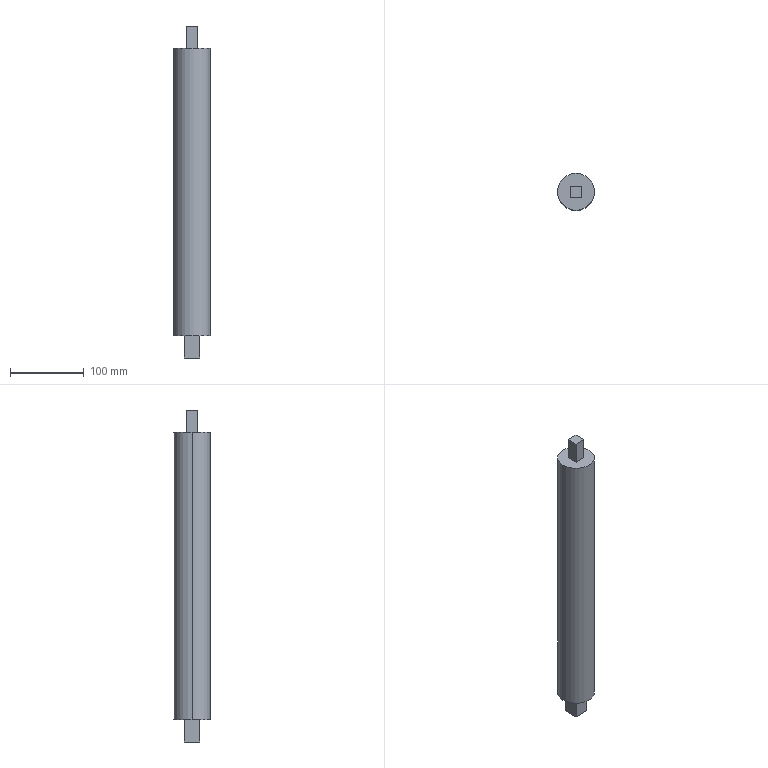Part | SolidWorks | features Extrusion 1, ICE 1, MoveFace 1 | 1 solid | 14 faces | box 50 x 50 x 450 mm | volume 785743 mm3 | plane 12 | cylinder 2 | commonest cylinder face diameters 50 x2
STEP:
#1=CARTESIAN_POINT('',(25.,0.,195.));
#2=VERTEX_POINT('',#1);
#3=CARTESIAN_POINT('',(-25.,0.,195.));
#4=VERTEX_POINT('',#3);
#5=CARTESIAN_POINT('',(0.,0.,195.));
#6=DIRECTION('',(0.,0.,1.));
#7=DIRECTION('',(1.,0.,0.));
#8=AXIS2_PLACEMENT_3D('',#5,#6,#7);
#9=CIRCLE('',#8,25.);
#10=EDGE_CURVE('',#2,#4,#9,.T.);
#11=ORIENTED_EDGE('',*,*,#10,.F.);
#12=CARTESIAN_POINT('',(25.,0.,-195.));
#13=VERTEX_POINT('',#12);
#14=CARTESIAN_POINT('',(25.,0.,195.));
#15=DIRECTION('',(0.,0.,-1.));
#16=VECTOR('',#15,1000.);
#17=LINE('',#14,#16);
#18=EDGE_CURVE('',#2,#13,#17,.T.);
#19=ORIENTED_EDGE('',*,*,#18,.T.);
#20=CARTESIAN_POINT('',(-25.,0.,-195.));
#21=VERTEX_POINT('',#20);
#22=CARTESIAN_POINT('',(0.,0.,-195.));
#23=DIRECTION('',(0.,0.,1.));
#24=DIRECTION('',(1.,0.,0.));
#25=AXIS2_PLACEMENT_3D('',#22,#23,#24);
#26=CIRCLE('',#25,25.);
#27=EDGE_CURVE('',#13,#21,#26,.T.);
#28=ORIENTED_EDGE('',*,*,#27,.T.);
#29=CARTESIAN_POINT('',(-25.,0.,195.));
#30=DIRECTION('',(0.,0.,-1.));
#31=VECTOR('',#30,1000.);
#32=LINE('',#29,#31);
#33=EDGE_CURVE('',#4,#21,#32,.T.);
#34=ORIENTED_EDGE('',*,*,#33,.F.);
#35=EDGE_LOOP('',(#11,#19,#28,#34));
#36=FACE_OUTER_BOUND('',#35,.T.);
#37=CARTESIAN_POINT('',(0.,0.,195.));
#38=DIRECTION('',(0.,0.,-1.));
#39=DIRECTION('',(-1.,0.,0.));
#40=AXIS2_PLACEMENT_3D('',#37,#38,#39);
#41=CYLINDRICAL_SURFACE('',#40,25.);
#42=ADVANCED_FACE('',(#36),#41,.T.);
#43=CARTESIAN_POINT('',(0.,0.,195.));
#44=DIRECTION('',(0.,0.,1.));
#45=DIRECTION('',(1.,0.,0.));
#46=AXIS2_PLACEMENT_3D('',#43,#44,#45);
#47=CIRCLE('',#46,25.);
#48=EDGE_CURVE('',#4,#2,#47,.T.);
#49=ORIENTED_EDGE('',*,*,#48,.T.);
#50=ORIENTED_EDGE('',*,*,#10,.T.);
#51=EDGE_LOOP('',(#49,#50));
#52=FACE_OUTER_BOUND('',#51,.T.);
#53=CARTESIAN_POINT('',(-7.5,7.5,195.));
#54=VERTEX_POINT('',#53);
#55=CARTESIAN_POINT('',(7.5,7.5,195.));
#56=VERTEX_POINT('',#55);
#57=CARTESIAN_POINT('',(0.,7.5,195.));
#58=DIRECTION('',(1.,0.,0.));
#59=VECTOR('',#58,1000.);
#60=LINE('',#57,#59);
#61=EDGE_CURVE('',#54,#56,#60,.T.);
#62=ORIENTED_EDGE('',*,*,#61,.T.);
#63=CARTESIAN_POINT('',(7.5,-7.5,195.));
#64=VERTEX_POINT('',#63);
#65=CARTESIAN_POINT('',(7.5,0.,195.));
#66=DIRECTION('',(0.,-1.,0.));
#67=VECTOR('',#66,1000.);
#68=LINE('',#65,#67);
#69=EDGE_CURVE('',#56,#64,#68,.T.);
#70=ORIENTED_EDGE('',*,*,#69,.T.);
#71=CARTESIAN_POINT('',(-7.5,-7.5,195.));
#72=VERTEX_POINT('',#71);
#73=CARTESIAN_POINT('',(0.,-7.5,195.));
#74=DIRECTION('',(-1.,0.,0.));
#75=VECTOR('',#74,1000.);
#76=LINE('',#73,#75);
#77=EDGE_CURVE('',#64,#72,#76,.T.);
#78=ORIENTED_EDGE('',*,*,#77,.T.);
#79=CARTESIAN_POINT('',(-7.5,0.,195.));
#80=DIRECTION('',(0.,1.,0.));
#81=VECTOR('',#80,1000.);
#82=LINE('',#79,#81);
#83=EDGE_CURVE('',#72,#54,#82,.T.);
#84=ORIENTED_EDGE('',*,*,#83,.T.);
#85=EDGE_LOOP('',(#62,#70,#78,#84));
#86=FACE_BOUND('',#85,.T.);
#87=CARTESIAN_POINT('',(0.,0.,195.));
#88=DIRECTION('',(0.,0.,1.));
#89=DIRECTION('',(1.,0.,0.));
#90=AXIS2_PLACEMENT_3D('',#87,#88,#89);
#91=PLANE('',#90);
#92=ADVANCED_FACE('',(#52,#86),#91,.T.);
#93=CARTESIAN_POINT('',(0.,0.,-195.));
#94=DIRECTION('',(0.,0.,1.));
#95=DIRECTION('',(1.,0.,0.));
#96=AXIS2_PLACEMENT_3D('',#93,#94,#95);
#97=CIRCLE('',#96,25.);
#98=EDGE_CURVE('',#21,#13,#97,.T.);
#99=ORIENTED_EDGE('',*,*,#98,.F.);
#100=ORIENTED_EDGE('',*,*,#27,.F.);
#101=EDGE_LOOP('',(#99,#100));
#102=FACE_OUTER_BOUND('',#101,.T.);
#103=CARTESIAN_POINT('',(10.5,10.5,-195.));
#104=VERTEX_POINT('',#103);
#105=CARTESIAN_POINT('',(10.5,-10.5,-195.));
#106=VERTEX_POINT('',#105);
#107=CARTESIAN_POINT('',(10.5,0.,-195.));
#108=DIRECTION('',(0.,-1.,0.));
#109=VECTOR('',#108,1000.);
#110=LINE('',#107,#109);
#111=EDGE_CURVE('',#104,#106,#110,.T.);
#112=ORIENTED_EDGE('',*,*,#111,.F.);
#113=CARTESIAN_POINT('',(-10.5,10.5,-195.));
#114=VERTEX_POINT('',#113);
#115=CARTESIAN_POINT('',(0.,10.5,-195.));
#116=DIRECTION('',(1.,0.,0.));
#117=VECTOR('',#116,1000.);
#118=LINE('',#115,#117);
#119=EDGE_CURVE('',#114,#104,#118,.T.);
#120=ORIENTED_EDGE('',*,*,#119,.F.);
#121=CARTESIAN_POINT('',(-10.5,-10.5,-195.));
#122=VERTEX_POINT('',#121);
#123=CARTESIAN_POINT('',(-10.5,0.,-195.));
#124=DIRECTION('',(0.,1.,0.));
#125=VECTOR('',#124,1000.);
#126=LINE('',#123,#125);
#127=EDGE_CURVE('',#122,#114,#126,.T.);
#128=ORIENTED_EDGE('',*,*,#127,.F.);
#129=CARTESIAN_POINT('',(0.,-10.5,-195.));
#130=DIRECTION('',(-1.,0.,0.));
#131=VECTOR('',#130,1000.);
#132=LINE('',#129,#131);
#133=EDGE_CURVE('',#106,#122,#132,.T.);
#134=ORIENTED_EDGE('',*,*,#133,.F.);
#135=EDGE_LOOP('',(#112,#120,#128,#134));
#136=FACE_BOUND('',#135,.T.);
#137=CARTESIAN_POINT('',(0.,0.,-195.));
#138=DIRECTION('',(0.,0.,1.));
#139=DIRECTION('',(1.,0.,0.));
#140=AXIS2_PLACEMENT_3D('',#137,#138,#139);
#141=PLANE('',#140);
#142=ADVANCED_FACE('',(#102,#136),#141,.F.);
#143=ORIENTED_EDGE('',*,*,#18,.F.);
#144=ORIENTED_EDGE('',*,*,#48,.F.);
#145=ORIENTED_EDGE('',*,*,#33,.T.);
#146=ORIENTED_EDGE('',*,*,#98,.T.);
#147=EDGE_LOOP('',(#143,#144,#145,#146));
#148=FACE_OUTER_BOUND('',#147,.T.);
#149=CARTESIAN_POINT('',(0.,0.,195.));
#150=DIRECTION('',(0.,0.,-1.));
#151=DIRECTION('',(-1.,0.,0.));
#152=AXIS2_PLACEMENT_3D('',#149,#150,#151);
#153=CYLINDRICAL_SURFACE('',#152,25.);
#154=ADVANCED_FACE('',(#148),#153,.T.);
#155=CARTESIAN_POINT('',(10.5,-10.5,-225.));
#156=VERTEX_POINT('',#155);
#157=CARTESIAN_POINT('',(10.5,10.5,-225.));
#158=VERTEX_POINT('',#157);
#159=CARTESIAN_POINT('',(10.5,7.5,-225.));
#160=DIRECTION('',(0.,1.,0.));
#161=VECTOR('',#160,1000.);
#162=LINE('',#159,#161);
#163=EDGE_CURVE('',#156,#158,#162,.T.);
#164=ORIENTED_EDGE('',*,*,#163,.F.);
#165=CARTESIAN_POINT('',(-10.5,-10.5,-225.));
#166=VERTEX_POINT('',#165);
#167=CARTESIAN_POINT('',(-7.5,-10.5,-225.));
#168=DIRECTION('',(1.,0.,0.));
#169=VECTOR('',#168,1000.);
#170=LINE('',#167,#169);
#171=EDGE_CURVE('',#166,#156,#170,.T.);
#172=ORIENTED_EDGE('',*,*,#171,.F.);
#173=CARTESIAN_POINT('',(-10.5,10.5,-225.));
#174=VERTEX_POINT('',#173);
#175=CARTESIAN_POINT('',(-10.5,7.5,-225.));
#176=DIRECTION('',(0.,-1.,0.));
#177=VECTOR('',#176,1000.);
#178=LINE('',#175,#177);
#179=EDGE_CURVE('',#174,#166,#178,.T.);
#180=ORIENTED_EDGE('',*,*,#179,.F.);
#181=CARTESIAN_POINT('',(-7.5,10.5,-225.));
#182=DIRECTION('',(-1.,0.,0.));
#183=VECTOR('',#182,1000.);
#184=LINE('',#181,#183);
#185=EDGE_CURVE('',#158,#174,#184,.T.);
#186=ORIENTED_EDGE('',*,*,#185,.F.);
#187=EDGE_LOOP('',(#164,#172,#180,#186));
#188=FACE_OUTER_BOUND('',#187,.T.);
#189=CARTESIAN_POINT('',(0.,0.,-225.));
#190=DIRECTION('',(0.,0.,1.));
#191=DIRECTION('',(1.,0.,0.));
#192=AXIS2_PLACEMENT_3D('',#189,#190,#191);
#193=PLANE('',#192);
#194=ADVANCED_FACE('',(#188),#193,.F.);
#195=CARTESIAN_POINT('',(10.5,-10.5,225.));
#196=DIRECTION('',(0.,0.,-1.));
#197=VECTOR('',#196,1000.);
#198=LINE('',#195,#197);
#199=EDGE_CURVE('',#106,#156,#198,.T.);
#200=ORIENTED_EDGE('',*,*,#199,.F.);
#201=ORIENTED_EDGE('',*,*,#133,.T.);
#202=CARTESIAN_POINT('',(-10.5,-10.5,225.));
#203=DIRECTION('',(0.,0.,-1.));
#204=VECTOR('',#203,1000.);
#205=LINE('',#202,#204);
#206=EDGE_CURVE('',#122,#166,#205,.T.);
#207=ORIENTED_EDGE('',*,*,#206,.T.);
#208=ORIENTED_EDGE('',*,*,#171,.T.);
#209=EDGE_LOOP('',(#200,#201,#207,#208));
#210=FACE_OUTER_BOUND('',#209,.T.);
#211=CARTESIAN_POINT('',(-7.5,-10.5,225.));
#212=DIRECTION('',(0.,1.,0.));
#213=DIRECTION('',(0.,0.,1.));
#214=AXIS2_PLACEMENT_3D('',#211,#212,#213);
#215=PLANE('',#214);
#216=ADVANCED_FACE('',(#210),#215,.F.);
#217=ORIENTED_EDGE('',*,*,#206,.F.);
#218=ORIENTED_EDGE('',*,*,#127,.T.);
#219=CARTESIAN_POINT('',(-10.5,10.5,225.));
#220=DIRECTION('',(0.,0.,-1.));
#221=VECTOR('',#220,1000.);
#222=LINE('',#219,#221);
#223=EDGE_CURVE('',#114,#174,#222,.T.);
#224=ORIENTED_EDGE('',*,*,#223,.T.);
#225=ORIENTED_EDGE('',*,*,#179,.T.);
#226=EDGE_LOOP('',(#217,#218,#224,#225));
#227=FACE_OUTER_BOUND('',#226,.T.);
#228=CARTESIAN_POINT('',(-10.5,7.5,225.));
#229=DIRECTION('',(1.,0.,0.));
#230=DIRECTION('',(0.,0.,-1.));
#231=AXIS2_PLACEMENT_3D('',#228,#229,#230);
#232=PLANE('',#231);
#233=ADVANCED_FACE('',(#227),#232,.F.);
#234=ORIENTED_EDGE('',*,*,#223,.F.);
#235=ORIENTED_EDGE('',*,*,#119,.T.);
#236=CARTESIAN_POINT('',(10.5,10.5,225.));
#237=DIRECTION('',(0.,0.,-1.));
#238=VECTOR('',#237,1000.);
#239=LINE('',#236,#238);
#240=EDGE_CURVE('',#104,#158,#239,.T.);
#241=ORIENTED_EDGE('',*,*,#240,.T.);
#242=ORIENTED_EDGE('',*,*,#185,.T.);
#243=EDGE_LOOP('',(#234,#235,#241,#242));
#244=FACE_OUTER_BOUND('',#243,.T.);
#245=CARTESIAN_POINT('',(-7.5,10.5,225.));
#246=DIRECTION('',(0.,-1.,0.));
#247=DIRECTION('',(0.,0.,-1.));
#248=AXIS2_PLACEMENT_3D('',#245,#246,#247);
#249=PLANE('',#248);
#250=ADVANCED_FACE('',(#244),#249,.F.);
#251=ORIENTED_EDGE('',*,*,#240,.F.);
#252=ORIENTED_EDGE('',*,*,#111,.T.);
#253=ORIENTED_EDGE('',*,*,#199,.T.);
#254=ORIENTED_EDGE('',*,*,#163,.T.);
#255=EDGE_LOOP('',(#251,#252,#253,#254));
#256=FACE_OUTER_BOUND('',#255,.T.);
#257=CARTESIAN_POINT('',(10.5,7.5,225.));
#258=DIRECTION('',(-1.,0.,0.));
#259=DIRECTION('',(0.,0.,1.));
#260=AXIS2_PLACEMENT_3D('',#257,#258,#259);
#261=PLANE('',#260);
#262=ADVANCED_FACE('',(#256),#261,.F.);
#263=ORIENTED_EDGE('',*,*,#69,.F.);
#264=CARTESIAN_POINT('',(7.5,7.5,225.));
#265=VERTEX_POINT('',#264);
#266=CARTESIAN_POINT('',(7.5,7.5,225.));
#267=DIRECTION('',(0.,0.,-1.));
#268=VECTOR('',#267,1000.);
#269=LINE('',#266,#268);
#270=EDGE_CURVE('',#265,#56,#269,.T.);
#271=ORIENTED_EDGE('',*,*,#270,.F.);
#272=CARTESIAN_POINT('',(7.5,-7.5,225.));
#273=VERTEX_POINT('',#272);
#274=CARTESIAN_POINT('',(7.5,7.5,225.));
#275=DIRECTION('',(0.,1.,0.));
#276=VECTOR('',#275,1000.);
#277=LINE('',#274,#276);
#278=EDGE_CURVE('',#273,#265,#277,.T.);
#279=ORIENTED_EDGE('',*,*,#278,.F.);
#280=CARTESIAN_POINT('',(7.5,-7.5,225.));
#281=DIRECTION('',(0.,0.,-1.));
#282=VECTOR('',#281,1000.);
#283=LINE('',#280,#282);
#284=EDGE_CURVE('',#273,#64,#283,.T.);
#285=ORIENTED_EDGE('',*,*,#284,.T.);
#286=EDGE_LOOP('',(#263,#271,#279,#285));
#287=FACE_OUTER_BOUND('',#286,.T.);
#288=CARTESIAN_POINT('',(7.5,7.5,225.));
#289=DIRECTION('',(-1.,0.,0.));
#290=DIRECTION('',(0.,0.,1.));
#291=AXIS2_PLACEMENT_3D('',#288,#289,#290);
#292=PLANE('',#291);
#293=ADVANCED_FACE('',(#287),#292,.F.);
#294=ORIENTED_EDGE('',*,*,#61,.F.);
#295=CARTESIAN_POINT('',(-7.5,7.5,225.));
#296=VERTEX_POINT('',#295);
#297=CARTESIAN_POINT('',(-7.5,7.5,225.));
#298=DIRECTION('',(0.,0.,-1.));
#299=VECTOR('',#298,1000.);
#300=LINE('',#297,#299);
#301=EDGE_CURVE('',#296,#54,#300,.T.);
#302=ORIENTED_EDGE('',*,*,#301,.F.);
#303=CARTESIAN_POINT('',(-7.5,7.5,225.));
#304=DIRECTION('',(-1.,0.,0.));
#305=VECTOR('',#304,1000.);
#306=LINE('',#303,#305);
#307=EDGE_CURVE('',#265,#296,#306,.T.);
#308=ORIENTED_EDGE('',*,*,#307,.F.);
#309=ORIENTED_EDGE('',*,*,#270,.T.);
#310=EDGE_LOOP('',(#294,#302,#308,#309));
#311=FACE_OUTER_BOUND('',#310,.T.);
#312=CARTESIAN_POINT('',(-7.5,7.5,225.));
#313=DIRECTION('',(0.,-1.,0.));
#314=DIRECTION('',(0.,0.,-1.));
#315=AXIS2_PLACEMENT_3D('',#312,#313,#314);
#316=PLANE('',#315);
#317=ADVANCED_FACE('',(#311),#316,.F.);
#318=ORIENTED_EDGE('',*,*,#83,.F.);
#319=CARTESIAN_POINT('',(-7.5,-7.5,225.));
#320=VERTEX_POINT('',#319);
#321=CARTESIAN_POINT('',(-7.5,-7.5,225.));
#322=DIRECTION('',(0.,0.,-1.));
#323=VECTOR('',#322,1000.);
#324=LINE('',#321,#323);
#325=EDGE_CURVE('',#320,#72,#324,.T.);
#326=ORIENTED_EDGE('',*,*,#325,.F.);
#327=CARTESIAN_POINT('',(-7.5,7.5,225.));
#328=DIRECTION('',(0.,-1.,0.));
#329=VECTOR('',#328,1000.);
#330=LINE('',#327,#329);
#331=EDGE_CURVE('',#296,#320,#330,.T.);
#332=ORIENTED_EDGE('',*,*,#331,.F.);
#333=ORIENTED_EDGE('',*,*,#301,.T.);
#334=EDGE_LOOP('',(#318,#326,#332,#333));
#335=FACE_OUTER_BOUND('',#334,.T.);
#336=CARTESIAN_POINT('',(-7.5,7.5,225.));
#337=DIRECTION('',(1.,0.,0.));
#338=DIRECTION('',(0.,0.,-1.));
#339=AXIS2_PLACEMENT_3D('',#336,#337,#338);
#340=PLANE('',#339);
#341=ADVANCED_FACE('',(#335),#340,.F.);
#342=ORIENTED_EDGE('',*,*,#77,.F.);
#343=ORIENTED_EDGE('',*,*,#284,.F.);
#344=CARTESIAN_POINT('',(-7.5,-7.5,225.));
#345=DIRECTION('',(1.,0.,0.));
#346=VECTOR('',#345,1000.);
#347=LINE('',#344,#346);
#348=EDGE_CURVE('',#320,#273,#347,.T.);
#349=ORIENTED_EDGE('',*,*,#348,.F.);
#350=ORIENTED_EDGE('',*,*,#325,.T.);
#351=EDGE_LOOP('',(#342,#343,#349,#350));
#352=FACE_OUTER_BOUND('',#351,.T.);
#353=CARTESIAN_POINT('',(-7.5,-7.5,225.));
#354=DIRECTION('',(0.,1.,0.));
#355=DIRECTION('',(0.,0.,1.));
#356=AXIS2_PLACEMENT_3D('',#353,#354,#355);
#357=PLANE('',#356);
#358=ADVANCED_FACE('',(#352),#357,.F.);
#359=ORIENTED_EDGE('',*,*,#278,.T.);
#360=ORIENTED_EDGE('',*,*,#307,.T.);
#361=ORIENTED_EDGE('',*,*,#331,.T.);
#362=ORIENTED_EDGE('',*,*,#348,.T.);
#363=EDGE_LOOP('',(#359,#360,#361,#362));
#364=FACE_OUTER_BOUND('',#363,.T.);
#365=CARTESIAN_POINT('',(0.,0.,225.));
#366=DIRECTION('',(0.,0.,1.));
#367=DIRECTION('',(1.,0.,0.));
#368=AXIS2_PLACEMENT_3D('',#365,#366,#367);
#369=PLANE('',#368);
#370=ADVANCED_FACE('',(#364),#369,.T.);
#371=CLOSED_SHELL('',(#42,#92,#142,#154,#194,#216,#233,#250,#262,#293,#317,#341,#358,#370));
#372=MANIFOLD_SOLID_BREP('',#371);
#373=CARTESIAN_POINT('',(0.,0.,0.));
#374=DIRECTION('',(0.,0.,1.));
#375=DIRECTION('',(1.,0.,0.));
#376=AXIS2_PLACEMENT_3D('',#373,#374,#375);
#377=(LENGTH_UNIT()NAMED_UNIT(*)SI_UNIT(.MILLI.,.METRE.));
#378=UNCERTAINTY_MEASURE_WITH_UNIT(LENGTH_MEASURE(0.00001),#377,'','');
#379=(NAMED_UNIT(*)PLANE_ANGLE_UNIT()SI_UNIT($,.RADIAN.));
#380=(NAMED_UNIT(*)SI_UNIT($,.STERADIAN.)SOLID_ANGLE_UNIT());
#381=(GEOMETRIC_REPRESENTATION_CONTEXT(3)GLOBAL_UNCERTAINTY_ASSIGNED_CONTEXT((#378))GLOBAL_UNIT_ASSIGNED_CONTEXT((#377,#379,#380))REPRESENTATION_CONTEXT('',''));
#382=ADVANCED_BREP_SHAPE_REPRESENTATION('',(#372,#376),#381);